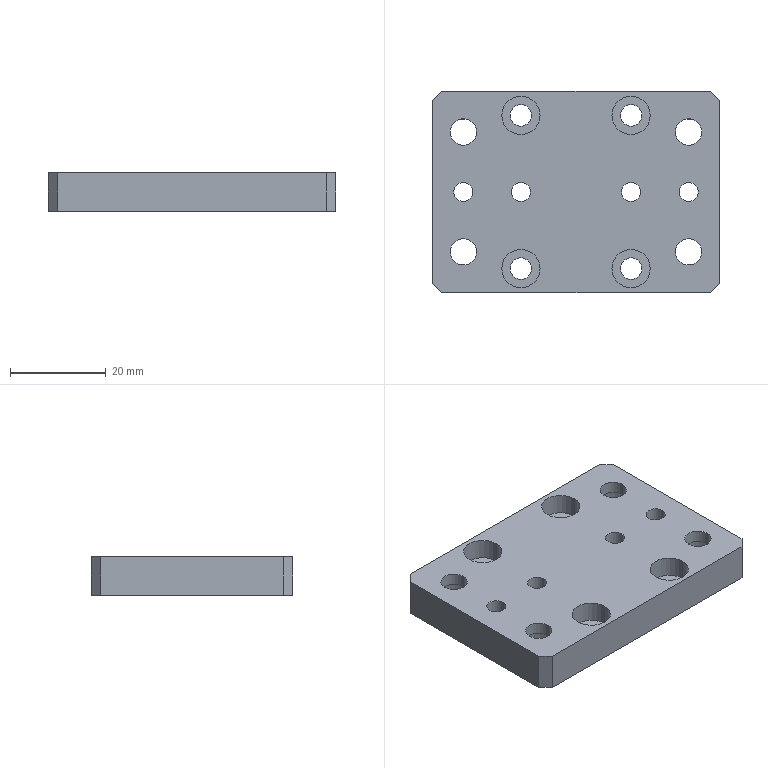Part | SolidWorks | features HoleWzd 2, ICE 2, Chamfer 1, Extrusion 1 | 1 solid | 58 faces | box 60 x 42 x 8 mm | volume 16637 mm3 | cylinder 40 | plane 18 | commonest cylinder face diameters 4 x8 4.5 x8 5.5 x8 8 x8 10 x8